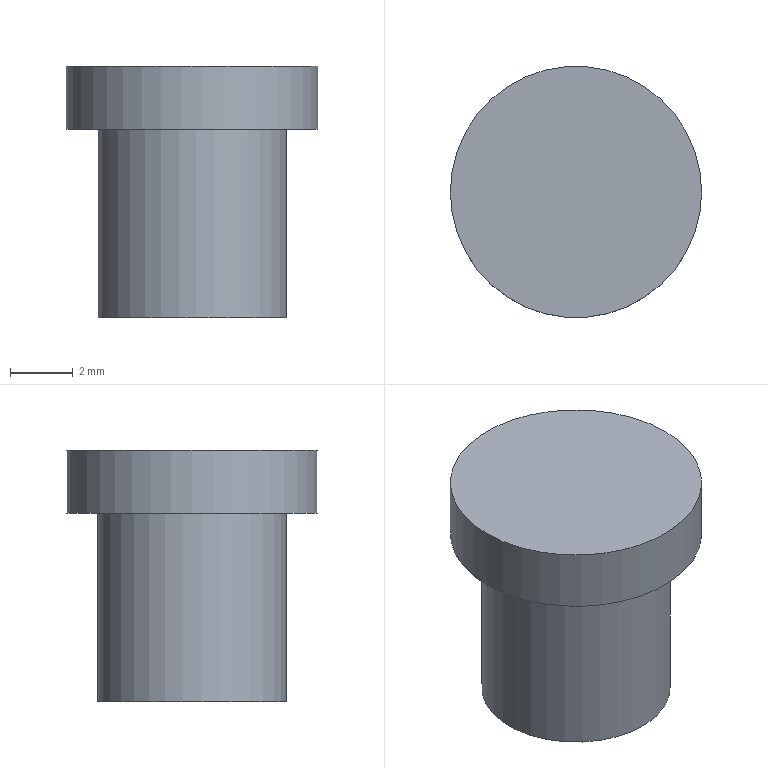Part | NX | features CYLINDER 2, DATUM_CSYS 1 | 1 solid | 5 faces | box 8 x 8 x 8 mm | volume 270.177 mm3 | plane 3 | cylinder 2 | commonest cylinder face diameters 6 x1 8 x1
STEP:
#1=CARTESIAN_POINT('',(3.,0.,0.));
#2=VERTEX_POINT('',#1);
#3=CARTESIAN_POINT('',(0.,0.,0.));
#4=DIRECTION('',(0.,0.,1.));
#5=DIRECTION('',(1.,0.,0.));
#6=AXIS2_PLACEMENT_3D('',#3,#4,#5);
#7=CIRCLE('',#6,3.);
#8=EDGE_CURVE('',#2,#2,#7,.T.);
#9=ORIENTED_EDGE('',*,*,#8,.F.);
#10=EDGE_LOOP('',(#9));
#11=FACE_BOUND('',#10,.T.);
#12=CARTESIAN_POINT('',(0.,0.,0.));
#13=DIRECTION('',(0.,0.,-1.));
#14=DIRECTION('',(-1.,0.,0.));
#15=AXIS2_PLACEMENT_3D('',#12,#13,#14);
#16=PLANE('',#15);
#17=ADVANCED_FACE('',(#11),#16,.T.);
#18=CARTESIAN_POINT('',(3.,0.,6.));
#19=VERTEX_POINT('',#18);
#20=CARTESIAN_POINT('',(0.,0.,6.));
#21=DIRECTION('',(0.,0.,-1.));
#22=DIRECTION('',(1.,0.,0.));
#23=AXIS2_PLACEMENT_3D('',#20,#21,#22);
#24=CIRCLE('',#23,3.);
#25=EDGE_CURVE('',#19,#19,#24,.T.);
#26=ORIENTED_EDGE('',*,*,#25,.T.);
#27=EDGE_LOOP('',(#26));
#28=FACE_BOUND('',#27,.T.);
#29=ORIENTED_EDGE('',*,*,#8,.T.);
#30=EDGE_LOOP('',(#29));
#31=FACE_BOUND('',#30,.T.);
#32=CARTESIAN_POINT('',(0.,0.,0.));
#33=DIRECTION('',(0.,0.,1.));
#34=DIRECTION('',(1.,0.,0.));
#35=AXIS2_PLACEMENT_3D('',#32,#33,#34);
#36=CYLINDRICAL_SURFACE('',#35,3.);
#37=ADVANCED_FACE('',(#28,#31),#36,.T.);
#38=CARTESIAN_POINT('',(4.,0.,8.));
#39=VERTEX_POINT('',#38);
#40=CARTESIAN_POINT('',(0.,0.,8.));
#41=DIRECTION('',(0.,0.,-1.));
#42=DIRECTION('',(1.,0.,0.));
#43=AXIS2_PLACEMENT_3D('',#40,#41,#42);
#44=CIRCLE('',#43,4.);
#45=EDGE_CURVE('',#39,#39,#44,.T.);
#46=ORIENTED_EDGE('',*,*,#45,.F.);
#47=EDGE_LOOP('',(#46));
#48=FACE_BOUND('',#47,.T.);
#49=CARTESIAN_POINT('',(0.,0.,8.));
#50=DIRECTION('',(0.,0.,1.));
#51=DIRECTION('',(1.,0.,0.));
#52=AXIS2_PLACEMENT_3D('',#49,#50,#51);
#53=PLANE('',#52);
#54=ADVANCED_FACE('',(#48),#53,.T.);
#55=ORIENTED_EDGE('',*,*,#25,.F.);
#56=EDGE_LOOP('',(#55));
#57=FACE_BOUND('',#56,.T.);
#58=CARTESIAN_POINT('',(4.,0.,6.));
#59=VERTEX_POINT('',#58);
#60=CARTESIAN_POINT('',(0.,0.,6.));
#61=DIRECTION('',(0.,0.,1.));
#62=DIRECTION('',(1.,0.,0.));
#63=AXIS2_PLACEMENT_3D('',#60,#61,#62);
#64=CIRCLE('',#63,4.);
#65=EDGE_CURVE('',#59,#59,#64,.T.);
#66=ORIENTED_EDGE('',*,*,#65,.F.);
#67=EDGE_LOOP('',(#66));
#68=FACE_BOUND('',#67,.T.);
#69=CARTESIAN_POINT('',(0.,0.,6.));
#70=DIRECTION('',(0.,0.,-1.));
#71=DIRECTION('',(-1.,0.,0.));
#72=AXIS2_PLACEMENT_3D('',#69,#70,#71);
#73=PLANE('',#72);
#74=ADVANCED_FACE('',(#57,#68),#73,.T.);
#75=ORIENTED_EDGE('',*,*,#45,.T.);
#76=EDGE_LOOP('',(#75));
#77=FACE_BOUND('',#76,.T.);
#78=ORIENTED_EDGE('',*,*,#65,.T.);
#79=EDGE_LOOP('',(#78));
#80=FACE_BOUND('',#79,.T.);
#81=CARTESIAN_POINT('',(0.,0.,6.));
#82=DIRECTION('',(0.,0.,1.));
#83=DIRECTION('',(1.,0.,0.));
#84=AXIS2_PLACEMENT_3D('',#81,#82,#83);
#85=CYLINDRICAL_SURFACE('',#84,4.);
#86=ADVANCED_FACE('',(#77,#80),#85,.T.);
#87=CLOSED_SHELL('',(#17,#37,#54,#74,#86));
#88=MANIFOLD_SOLID_BREP('',#87);
#89=(LENGTH_UNIT()NAMED_UNIT(*)SI_UNIT(.MILLI.,.METRE.));
#90=UNCERTAINTY_MEASURE_WITH_UNIT(LENGTH_MEASURE(0.00001),#89,'','');
#91=(NAMED_UNIT(*)PLANE_ANGLE_UNIT()SI_UNIT($,.RADIAN.));
#92=(NAMED_UNIT(*)SI_UNIT($,.STERADIAN.)SOLID_ANGLE_UNIT());
#93=(GEOMETRIC_REPRESENTATION_CONTEXT(3)GLOBAL_UNCERTAINTY_ASSIGNED_CONTEXT((#90))GLOBAL_UNIT_ASSIGNED_CONTEXT((#89,#91,#92))REPRESENTATION_CONTEXT('',''));
#94=ADVANCED_BREP_SHAPE_REPRESENTATION('',(#88),#93);